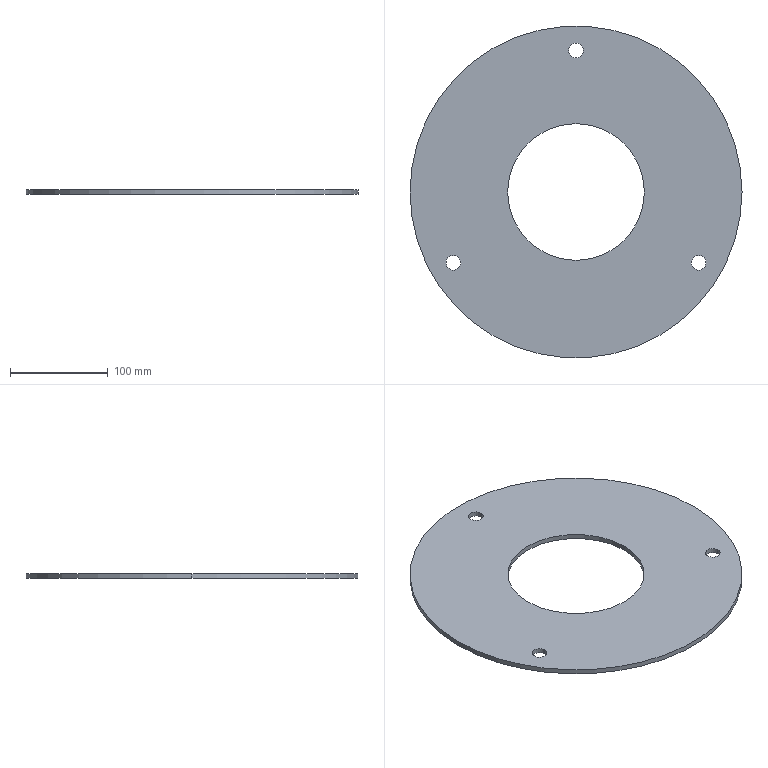Part | SolidWorks | features BaseBody 1 | 1 solid | 12 faces | box 340 x 340 x 5 mm | volume 374340 mm3 | cylinder 10 | plane 2 | commonest cylinder face diameters 15 x6 140 x2 340 x2
STEP:
#1=CARTESIAN_POINT('',(383.151,880.749,-639.893));
#2=VERTEX_POINT('',#1);
#3=CARTESIAN_POINT('',(383.151,880.749,-644.893));
#4=VERTEX_POINT('',#3);
#5=CARTESIAN_POINT('',(383.151,880.749,-644.893));
#6=DIRECTION('',(0.,0.,-1.));
#7=VECTOR('',#6,1000.);
#8=LINE('',#5,#7);
#9=EDGE_CURVE('',#2,#4,#8,.T.);
#10=ORIENTED_EDGE('',*,*,#9,.T.);
#11=CARTESIAN_POINT('',(398.151,880.749,-644.893));
#12=VERTEX_POINT('',#11);
#13=CARTESIAN_POINT('',(390.651,880.749,-644.893));
#14=DIRECTION('',(0.,0.,-1.));
#15=DIRECTION('',(-1.,0.,0.));
#16=AXIS2_PLACEMENT_3D('',#13,#14,#15);
#17=CIRCLE('',#16,7.5);
#18=EDGE_CURVE('',#4,#12,#17,.T.);
#19=ORIENTED_EDGE('',*,*,#18,.T.);
#20=CARTESIAN_POINT('',(398.151,880.749,-639.893));
#21=VERTEX_POINT('',#20);
#22=CARTESIAN_POINT('',(398.151,880.749,-644.893));
#23=DIRECTION('',(0.,0.,-1.));
#24=VECTOR('',#23,1000.);
#25=LINE('',#22,#24);
#26=EDGE_CURVE('',#21,#12,#25,.T.);
#27=ORIENTED_EDGE('',*,*,#26,.F.);
#28=CARTESIAN_POINT('',(390.651,880.749,-639.893));
#29=DIRECTION('',(0.,0.,-1.));
#30=DIRECTION('',(-1.,0.,0.));
#31=AXIS2_PLACEMENT_3D('',#28,#29,#30);
#32=CIRCLE('',#31,7.5);
#33=EDGE_CURVE('',#2,#21,#32,.T.);
#34=ORIENTED_EDGE('',*,*,#33,.F.);
#35=EDGE_LOOP('',(#10,#19,#27,#34));
#36=FACE_OUTER_BOUND('',#35,.T.);
#37=CARTESIAN_POINT('',(390.651,880.749,-644.893));
#38=DIRECTION('',(0.,0.,1.));
#39=DIRECTION('',(-1.,0.,0.));
#40=AXIS2_PLACEMENT_3D('',#37,#38,#39);
#41=CYLINDRICAL_SURFACE('',#40,7.5);
#42=ADVANCED_FACE('',(#36),#41,.F.);
#43=CARTESIAN_POINT('',(132.003,880.749,-639.893));
#44=VERTEX_POINT('',#43);
#45=CARTESIAN_POINT('',(132.003,880.749,-644.893));
#46=VERTEX_POINT('',#45);
#47=CARTESIAN_POINT('',(132.003,880.749,-644.893));
#48=DIRECTION('',(0.,0.,-1.));
#49=VECTOR('',#48,1000.);
#50=LINE('',#47,#49);
#51=EDGE_CURVE('',#44,#46,#50,.T.);
#52=ORIENTED_EDGE('',*,*,#51,.T.);
#53=CARTESIAN_POINT('',(147.003,880.749,-644.893));
#54=VERTEX_POINT('',#53);
#55=CARTESIAN_POINT('',(139.503,880.749,-644.893));
#56=DIRECTION('',(0.,0.,-1.));
#57=DIRECTION('',(-1.,0.,0.));
#58=AXIS2_PLACEMENT_3D('',#55,#56,#57);
#59=CIRCLE('',#58,7.5);
#60=EDGE_CURVE('',#46,#54,#59,.T.);
#61=ORIENTED_EDGE('',*,*,#60,.T.);
#62=CARTESIAN_POINT('',(147.003,880.749,-639.893));
#63=VERTEX_POINT('',#62);
#64=CARTESIAN_POINT('',(147.003,880.749,-644.893));
#65=DIRECTION('',(0.,0.,-1.));
#66=VECTOR('',#65,1000.);
#67=LINE('',#64,#66);
#68=EDGE_CURVE('',#63,#54,#67,.T.);
#69=ORIENTED_EDGE('',*,*,#68,.F.);
#70=CARTESIAN_POINT('',(139.503,880.749,-639.893));
#71=DIRECTION('',(0.,0.,-1.));
#72=DIRECTION('',(-1.,0.,0.));
#73=AXIS2_PLACEMENT_3D('',#70,#71,#72);
#74=CIRCLE('',#73,7.5);
#75=EDGE_CURVE('',#44,#63,#74,.T.);
#76=ORIENTED_EDGE('',*,*,#75,.F.);
#77=EDGE_LOOP('',(#52,#61,#69,#76));
#78=FACE_OUTER_BOUND('',#77,.T.);
#79=CARTESIAN_POINT('',(139.503,880.749,-644.893));
#80=DIRECTION('',(0.,0.,1.));
#81=DIRECTION('',(-1.,0.,0.));
#82=AXIS2_PLACEMENT_3D('',#79,#80,#81);
#83=CYLINDRICAL_SURFACE('',#82,7.5);
#84=ADVANCED_FACE('',(#78),#83,.F.);
#85=CARTESIAN_POINT('',(257.577,1098.249,-639.893));
#86=VERTEX_POINT('',#85);
#87=CARTESIAN_POINT('',(257.577,1098.249,-644.893));
#88=VERTEX_POINT('',#87);
#89=CARTESIAN_POINT('',(257.577,1098.249,-644.893));
#90=DIRECTION('',(0.,0.,-1.));
#91=VECTOR('',#90,1000.);
#92=LINE('',#89,#91);
#93=EDGE_CURVE('',#86,#88,#92,.T.);
#94=ORIENTED_EDGE('',*,*,#93,.T.);
#95=CARTESIAN_POINT('',(272.577,1098.249,-644.893));
#96=VERTEX_POINT('',#95);
#97=CARTESIAN_POINT('',(265.077,1098.249,-644.893));
#98=DIRECTION('',(0.,0.,-1.));
#99=DIRECTION('',(-1.,0.,0.));
#100=AXIS2_PLACEMENT_3D('',#97,#98,#99);
#101=CIRCLE('',#100,7.5);
#102=EDGE_CURVE('',#88,#96,#101,.T.);
#103=ORIENTED_EDGE('',*,*,#102,.T.);
#104=CARTESIAN_POINT('',(272.577,1098.249,-639.893));
#105=VERTEX_POINT('',#104);
#106=CARTESIAN_POINT('',(272.577,1098.249,-644.893));
#107=DIRECTION('',(0.,0.,-1.));
#108=VECTOR('',#107,1000.);
#109=LINE('',#106,#108);
#110=EDGE_CURVE('',#105,#96,#109,.T.);
#111=ORIENTED_EDGE('',*,*,#110,.F.);
#112=CARTESIAN_POINT('',(265.077,1098.249,-639.893));
#113=DIRECTION('',(0.,0.,-1.));
#114=DIRECTION('',(-1.,0.,0.));
#115=AXIS2_PLACEMENT_3D('',#112,#113,#114);
#116=CIRCLE('',#115,7.5);
#117=EDGE_CURVE('',#86,#105,#116,.T.);
#118=ORIENTED_EDGE('',*,*,#117,.F.);
#119=EDGE_LOOP('',(#94,#103,#111,#118));
#120=FACE_OUTER_BOUND('',#119,.T.);
#121=CARTESIAN_POINT('',(265.077,1098.249,-644.893));
#122=DIRECTION('',(0.,0.,1.));
#123=DIRECTION('',(-1.,0.,0.));
#124=AXIS2_PLACEMENT_3D('',#121,#122,#123);
#125=CYLINDRICAL_SURFACE('',#124,7.5);
#126=ADVANCED_FACE('',(#120),#125,.F.);
#127=CARTESIAN_POINT('',(195.077,953.249,-639.893));
#128=VERTEX_POINT('',#127);
#129=CARTESIAN_POINT('',(195.077,953.249,-644.893));
#130=VERTEX_POINT('',#129);
#131=CARTESIAN_POINT('',(195.077,953.249,-644.893));
#132=DIRECTION('',(0.,0.,-1.));
#133=VECTOR('',#132,1000.);
#134=LINE('',#131,#133);
#135=EDGE_CURVE('',#128,#130,#134,.T.);
#136=ORIENTED_EDGE('',*,*,#135,.T.);
#137=CARTESIAN_POINT('',(335.077,953.249,-644.893));
#138=VERTEX_POINT('',#137);
#139=CARTESIAN_POINT('',(265.077,953.249,-644.893));
#140=DIRECTION('',(0.,0.,-1.));
#141=DIRECTION('',(-1.,0.,0.));
#142=AXIS2_PLACEMENT_3D('',#139,#140,#141);
#143=CIRCLE('',#142,70.);
#144=EDGE_CURVE('',#130,#138,#143,.T.);
#145=ORIENTED_EDGE('',*,*,#144,.T.);
#146=CARTESIAN_POINT('',(335.077,953.249,-639.893));
#147=VERTEX_POINT('',#146);
#148=CARTESIAN_POINT('',(335.077,953.249,-644.893));
#149=DIRECTION('',(0.,0.,-1.));
#150=VECTOR('',#149,1000.);
#151=LINE('',#148,#150);
#152=EDGE_CURVE('',#147,#138,#151,.T.);
#153=ORIENTED_EDGE('',*,*,#152,.F.);
#154=CARTESIAN_POINT('',(265.077,953.249,-639.893));
#155=DIRECTION('',(0.,0.,-1.));
#156=DIRECTION('',(-1.,0.,0.));
#157=AXIS2_PLACEMENT_3D('',#154,#155,#156);
#158=CIRCLE('',#157,70.);
#159=EDGE_CURVE('',#128,#147,#158,.T.);
#160=ORIENTED_EDGE('',*,*,#159,.F.);
#161=EDGE_LOOP('',(#136,#145,#153,#160));
#162=FACE_OUTER_BOUND('',#161,.T.);
#163=CARTESIAN_POINT('',(265.077,953.249,-644.893));
#164=DIRECTION('',(0.,0.,1.));
#165=DIRECTION('',(-1.,0.,0.));
#166=AXIS2_PLACEMENT_3D('',#163,#164,#165);
#167=CYLINDRICAL_SURFACE('',#166,70.);
#168=ADVANCED_FACE('',(#162),#167,.F.);
#169=CARTESIAN_POINT('',(95.077,953.249,-639.893));
#170=VERTEX_POINT('',#169);
#171=CARTESIAN_POINT('',(95.077,953.249,-644.893));
#172=VERTEX_POINT('',#171);
#173=CARTESIAN_POINT('',(95.077,953.249,-644.893));
#174=DIRECTION('',(0.,0.,-1.));
#175=VECTOR('',#174,1000.);
#176=LINE('',#173,#175);
#177=EDGE_CURVE('',#170,#172,#176,.T.);
#178=ORIENTED_EDGE('',*,*,#177,.T.);
#179=CARTESIAN_POINT('',(435.077,953.249,-644.893));
#180=VERTEX_POINT('',#179);
#181=CARTESIAN_POINT('',(265.077,953.249,-644.893));
#182=DIRECTION('',(0.,0.,-1.));
#183=DIRECTION('',(-1.,0.,0.));
#184=AXIS2_PLACEMENT_3D('',#181,#182,#183);
#185=CIRCLE('',#184,170.);
#186=EDGE_CURVE('',#180,#172,#185,.T.);
#187=ORIENTED_EDGE('',*,*,#186,.F.);
#188=CARTESIAN_POINT('',(435.077,953.249,-639.893));
#189=VERTEX_POINT('',#188);
#190=CARTESIAN_POINT('',(435.077,953.249,-644.893));
#191=DIRECTION('',(0.,0.,-1.));
#192=VECTOR('',#191,1000.);
#193=LINE('',#190,#192);
#194=EDGE_CURVE('',#189,#180,#193,.T.);
#195=ORIENTED_EDGE('',*,*,#194,.F.);
#196=CARTESIAN_POINT('',(265.077,953.249,-639.893));
#197=DIRECTION('',(0.,0.,-1.));
#198=DIRECTION('',(-1.,0.,0.));
#199=AXIS2_PLACEMENT_3D('',#196,#197,#198);
#200=CIRCLE('',#199,170.);
#201=EDGE_CURVE('',#189,#170,#200,.T.);
#202=ORIENTED_EDGE('',*,*,#201,.T.);
#203=EDGE_LOOP('',(#178,#187,#195,#202));
#204=FACE_OUTER_BOUND('',#203,.T.);
#205=CARTESIAN_POINT('',(265.077,953.249,-644.893));
#206=DIRECTION('',(0.,0.,1.));
#207=DIRECTION('',(-1.,0.,0.));
#208=AXIS2_PLACEMENT_3D('',#205,#206,#207);
#209=CYLINDRICAL_SURFACE('',#208,170.);
#210=ADVANCED_FACE('',(#204),#209,.T.);
#211=CARTESIAN_POINT('',(390.651,880.749,-639.893));
#212=DIRECTION('',(0.,0.,-1.));
#213=DIRECTION('',(-1.,0.,0.));
#214=AXIS2_PLACEMENT_3D('',#211,#212,#213);
#215=CIRCLE('',#214,7.5);
#216=EDGE_CURVE('',#21,#2,#215,.T.);
#217=ORIENTED_EDGE('',*,*,#216,.T.);
#218=ORIENTED_EDGE('',*,*,#33,.T.);
#219=EDGE_LOOP('',(#217,#218));
#220=FACE_BOUND('',#219,.T.);
#221=CARTESIAN_POINT('',(265.077,1098.249,-639.893));
#222=DIRECTION('',(0.,0.,-1.));
#223=DIRECTION('',(-1.,0.,0.));
#224=AXIS2_PLACEMENT_3D('',#221,#222,#223);
#225=CIRCLE('',#224,7.5);
#226=EDGE_CURVE('',#105,#86,#225,.T.);
#227=ORIENTED_EDGE('',*,*,#226,.T.);
#228=ORIENTED_EDGE('',*,*,#117,.T.);
#229=EDGE_LOOP('',(#227,#228));
#230=FACE_BOUND('',#229,.T.);
#231=CARTESIAN_POINT('',(265.077,953.249,-639.893));
#232=DIRECTION('',(0.,0.,-1.));
#233=DIRECTION('',(-1.,0.,0.));
#234=AXIS2_PLACEMENT_3D('',#231,#232,#233);
#235=CIRCLE('',#234,70.);
#236=EDGE_CURVE('',#147,#128,#235,.T.);
#237=ORIENTED_EDGE('',*,*,#236,.T.);
#238=ORIENTED_EDGE('',*,*,#159,.T.);
#239=EDGE_LOOP('',(#237,#238));
#240=FACE_BOUND('',#239,.T.);
#241=CARTESIAN_POINT('',(139.503,880.749,-639.893));
#242=DIRECTION('',(0.,0.,-1.));
#243=DIRECTION('',(-1.,0.,0.));
#244=AXIS2_PLACEMENT_3D('',#241,#242,#243);
#245=CIRCLE('',#244,7.5);
#246=EDGE_CURVE('',#63,#44,#245,.T.);
#247=ORIENTED_EDGE('',*,*,#246,.T.);
#248=ORIENTED_EDGE('',*,*,#75,.T.);
#249=EDGE_LOOP('',(#247,#248));
#250=FACE_BOUND('',#249,.T.);
#251=ORIENTED_EDGE('',*,*,#201,.F.);
#252=CARTESIAN_POINT('',(265.077,953.249,-639.893));
#253=DIRECTION('',(0.,0.,-1.));
#254=DIRECTION('',(-1.,0.,0.));
#255=AXIS2_PLACEMENT_3D('',#252,#253,#254);
#256=CIRCLE('',#255,170.);
#257=EDGE_CURVE('',#170,#189,#256,.T.);
#258=ORIENTED_EDGE('',*,*,#257,.F.);
#259=EDGE_LOOP('',(#251,#258));
#260=FACE_OUTER_BOUND('',#259,.T.);
#261=CARTESIAN_POINT('',(265.077,953.249,-639.893));
#262=DIRECTION('',(0.,0.,-1.));
#263=DIRECTION('',(0.,-1.,0.));
#264=AXIS2_PLACEMENT_3D('',#261,#262,#263);
#265=PLANE('',#264);
#266=ADVANCED_FACE('',(#220,#230,#240,#250,#260),#265,.F.);
#267=CARTESIAN_POINT('',(390.651,880.749,-644.893));
#268=DIRECTION('',(0.,0.,-1.));
#269=DIRECTION('',(-1.,0.,0.));
#270=AXIS2_PLACEMENT_3D('',#267,#268,#269);
#271=CIRCLE('',#270,7.5);
#272=EDGE_CURVE('',#12,#4,#271,.T.);
#273=ORIENTED_EDGE('',*,*,#272,.F.);
#274=ORIENTED_EDGE('',*,*,#18,.F.);
#275=EDGE_LOOP('',(#273,#274));
#276=FACE_BOUND('',#275,.T.);
#277=CARTESIAN_POINT('',(265.077,1098.249,-644.893));
#278=DIRECTION('',(0.,0.,-1.));
#279=DIRECTION('',(-1.,0.,0.));
#280=AXIS2_PLACEMENT_3D('',#277,#278,#279);
#281=CIRCLE('',#280,7.5);
#282=EDGE_CURVE('',#96,#88,#281,.T.);
#283=ORIENTED_EDGE('',*,*,#282,.F.);
#284=ORIENTED_EDGE('',*,*,#102,.F.);
#285=EDGE_LOOP('',(#283,#284));
#286=FACE_BOUND('',#285,.T.);
#287=CARTESIAN_POINT('',(265.077,953.249,-644.893));
#288=DIRECTION('',(0.,0.,-1.));
#289=DIRECTION('',(-1.,0.,0.));
#290=AXIS2_PLACEMENT_3D('',#287,#288,#289);
#291=CIRCLE('',#290,70.);
#292=EDGE_CURVE('',#138,#130,#291,.T.);
#293=ORIENTED_EDGE('',*,*,#292,.F.);
#294=ORIENTED_EDGE('',*,*,#144,.F.);
#295=EDGE_LOOP('',(#293,#294));
#296=FACE_BOUND('',#295,.T.);
#297=CARTESIAN_POINT('',(139.503,880.749,-644.893));
#298=DIRECTION('',(0.,0.,-1.));
#299=DIRECTION('',(-1.,0.,0.));
#300=AXIS2_PLACEMENT_3D('',#297,#298,#299);
#301=CIRCLE('',#300,7.5);
#302=EDGE_CURVE('',#54,#46,#301,.T.);
#303=ORIENTED_EDGE('',*,*,#302,.F.);
#304=ORIENTED_EDGE('',*,*,#60,.F.);
#305=EDGE_LOOP('',(#303,#304));
#306=FACE_BOUND('',#305,.T.);
#307=ORIENTED_EDGE('',*,*,#186,.T.);
#308=CARTESIAN_POINT('',(265.077,953.249,-644.893));
#309=DIRECTION('',(0.,0.,-1.));
#310=DIRECTION('',(-1.,0.,0.));
#311=AXIS2_PLACEMENT_3D('',#308,#309,#310);
#312=CIRCLE('',#311,170.);
#313=EDGE_CURVE('',#172,#180,#312,.T.);
#314=ORIENTED_EDGE('',*,*,#313,.T.);
#315=EDGE_LOOP('',(#307,#314));
#316=FACE_OUTER_BOUND('',#315,.T.);
#317=CARTESIAN_POINT('',(265.077,953.249,-644.893));
#318=DIRECTION('',(0.,0.,-1.));
#319=DIRECTION('',(0.,-1.,0.));
#320=AXIS2_PLACEMENT_3D('',#317,#318,#319);
#321=PLANE('',#320);
#322=ADVANCED_FACE('',(#276,#286,#296,#306,#316),#321,.T.);
#323=ORIENTED_EDGE('',*,*,#313,.F.);
#324=ORIENTED_EDGE('',*,*,#177,.F.);
#325=ORIENTED_EDGE('',*,*,#257,.T.);
#326=ORIENTED_EDGE('',*,*,#194,.T.);
#327=EDGE_LOOP('',(#323,#324,#325,#326));
#328=FACE_OUTER_BOUND('',#327,.T.);
#329=CARTESIAN_POINT('',(265.077,953.249,-644.893));
#330=DIRECTION('',(0.,0.,1.));
#331=DIRECTION('',(-1.,0.,0.));
#332=AXIS2_PLACEMENT_3D('',#329,#330,#331);
#333=CYLINDRICAL_SURFACE('',#332,170.);
#334=ADVANCED_FACE('',(#328),#333,.T.);
#335=ORIENTED_EDGE('',*,*,#292,.T.);
#336=ORIENTED_EDGE('',*,*,#135,.F.);
#337=ORIENTED_EDGE('',*,*,#236,.F.);
#338=ORIENTED_EDGE('',*,*,#152,.T.);
#339=EDGE_LOOP('',(#335,#336,#337,#338));
#340=FACE_OUTER_BOUND('',#339,.T.);
#341=CARTESIAN_POINT('',(265.077,953.249,-644.893));
#342=DIRECTION('',(0.,0.,1.));
#343=DIRECTION('',(-1.,0.,0.));
#344=AXIS2_PLACEMENT_3D('',#341,#342,#343);
#345=CYLINDRICAL_SURFACE('',#344,70.);
#346=ADVANCED_FACE('',(#340),#345,.F.);
#347=ORIENTED_EDGE('',*,*,#282,.T.);
#348=ORIENTED_EDGE('',*,*,#93,.F.);
#349=ORIENTED_EDGE('',*,*,#226,.F.);
#350=ORIENTED_EDGE('',*,*,#110,.T.);
#351=EDGE_LOOP('',(#347,#348,#349,#350));
#352=FACE_OUTER_BOUND('',#351,.T.);
#353=CARTESIAN_POINT('',(265.077,1098.249,-644.893));
#354=DIRECTION('',(0.,0.,1.));
#355=DIRECTION('',(-1.,0.,0.));
#356=AXIS2_PLACEMENT_3D('',#353,#354,#355);
#357=CYLINDRICAL_SURFACE('',#356,7.5);
#358=ADVANCED_FACE('',(#352),#357,.F.);
#359=ORIENTED_EDGE('',*,*,#302,.T.);
#360=ORIENTED_EDGE('',*,*,#51,.F.);
#361=ORIENTED_EDGE('',*,*,#246,.F.);
#362=ORIENTED_EDGE('',*,*,#68,.T.);
#363=EDGE_LOOP('',(#359,#360,#361,#362));
#364=FACE_OUTER_BOUND('',#363,.T.);
#365=CARTESIAN_POINT('',(139.503,880.749,-644.893));
#366=DIRECTION('',(0.,0.,1.));
#367=DIRECTION('',(-1.,0.,0.));
#368=AXIS2_PLACEMENT_3D('',#365,#366,#367);
#369=CYLINDRICAL_SURFACE('',#368,7.5);
#370=ADVANCED_FACE('',(#364),#369,.F.);
#371=ORIENTED_EDGE('',*,*,#272,.T.);
#372=ORIENTED_EDGE('',*,*,#9,.F.);
#373=ORIENTED_EDGE('',*,*,#216,.F.);
#374=ORIENTED_EDGE('',*,*,#26,.T.);
#375=EDGE_LOOP('',(#371,#372,#373,#374));
#376=FACE_OUTER_BOUND('',#375,.T.);
#377=CARTESIAN_POINT('',(390.651,880.749,-644.893));
#378=DIRECTION('',(0.,0.,1.));
#379=DIRECTION('',(-1.,0.,0.));
#380=AXIS2_PLACEMENT_3D('',#377,#378,#379);
#381=CYLINDRICAL_SURFACE('',#380,7.5);
#382=ADVANCED_FACE('',(#376),#381,.F.);
#383=CLOSED_SHELL('',(#42,#84,#126,#168,#210,#266,#322,#334,#346,#358,#370,#382));
#384=MANIFOLD_SOLID_BREP('',#383);
#385=CARTESIAN_POINT('',(0.,0.,0.));
#386=DIRECTION('',(0.,0.,1.));
#387=DIRECTION('',(1.,0.,0.));
#388=AXIS2_PLACEMENT_3D('',#385,#386,#387);
#389=(LENGTH_UNIT()NAMED_UNIT(*)SI_UNIT(.MILLI.,.METRE.));
#390=UNCERTAINTY_MEASURE_WITH_UNIT(LENGTH_MEASURE(0.00001),#389,'','');
#391=(NAMED_UNIT(*)PLANE_ANGLE_UNIT()SI_UNIT($,.RADIAN.));
#392=(NAMED_UNIT(*)SI_UNIT($,.STERADIAN.)SOLID_ANGLE_UNIT());
#393=(GEOMETRIC_REPRESENTATION_CONTEXT(3)GLOBAL_UNCERTAINTY_ASSIGNED_CONTEXT((#390))GLOBAL_UNIT_ASSIGNED_CONTEXT((#389,#391,#392))REPRESENTATION_CONTEXT('',''));
#394=ADVANCED_BREP_SHAPE_REPRESENTATION('',(#384,#388),#393);